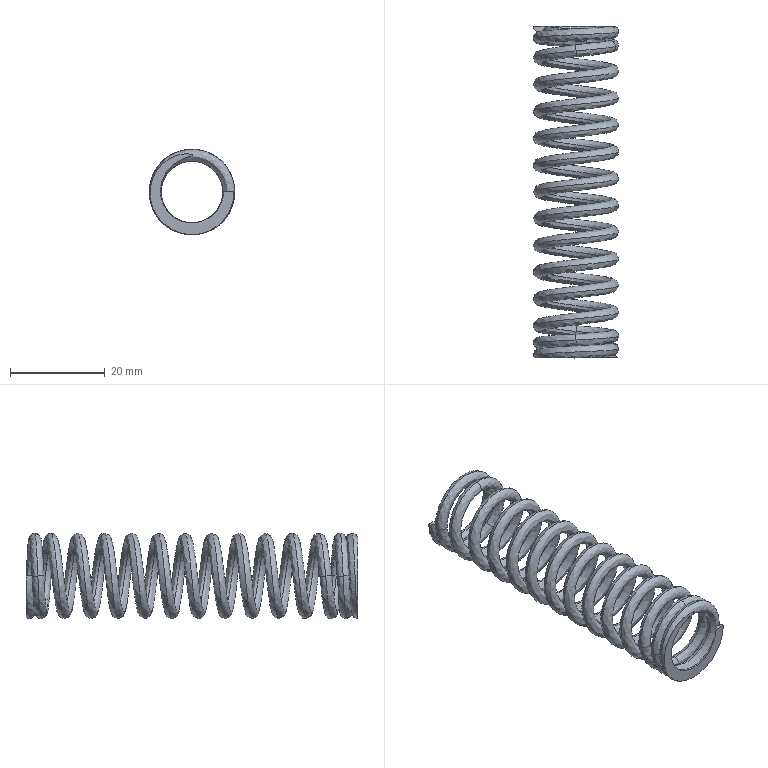Part | STEP file | Compress Spring1_4 | 1 solid | 26 faces | volume 3363 mm3 | spline 22 | plane 4